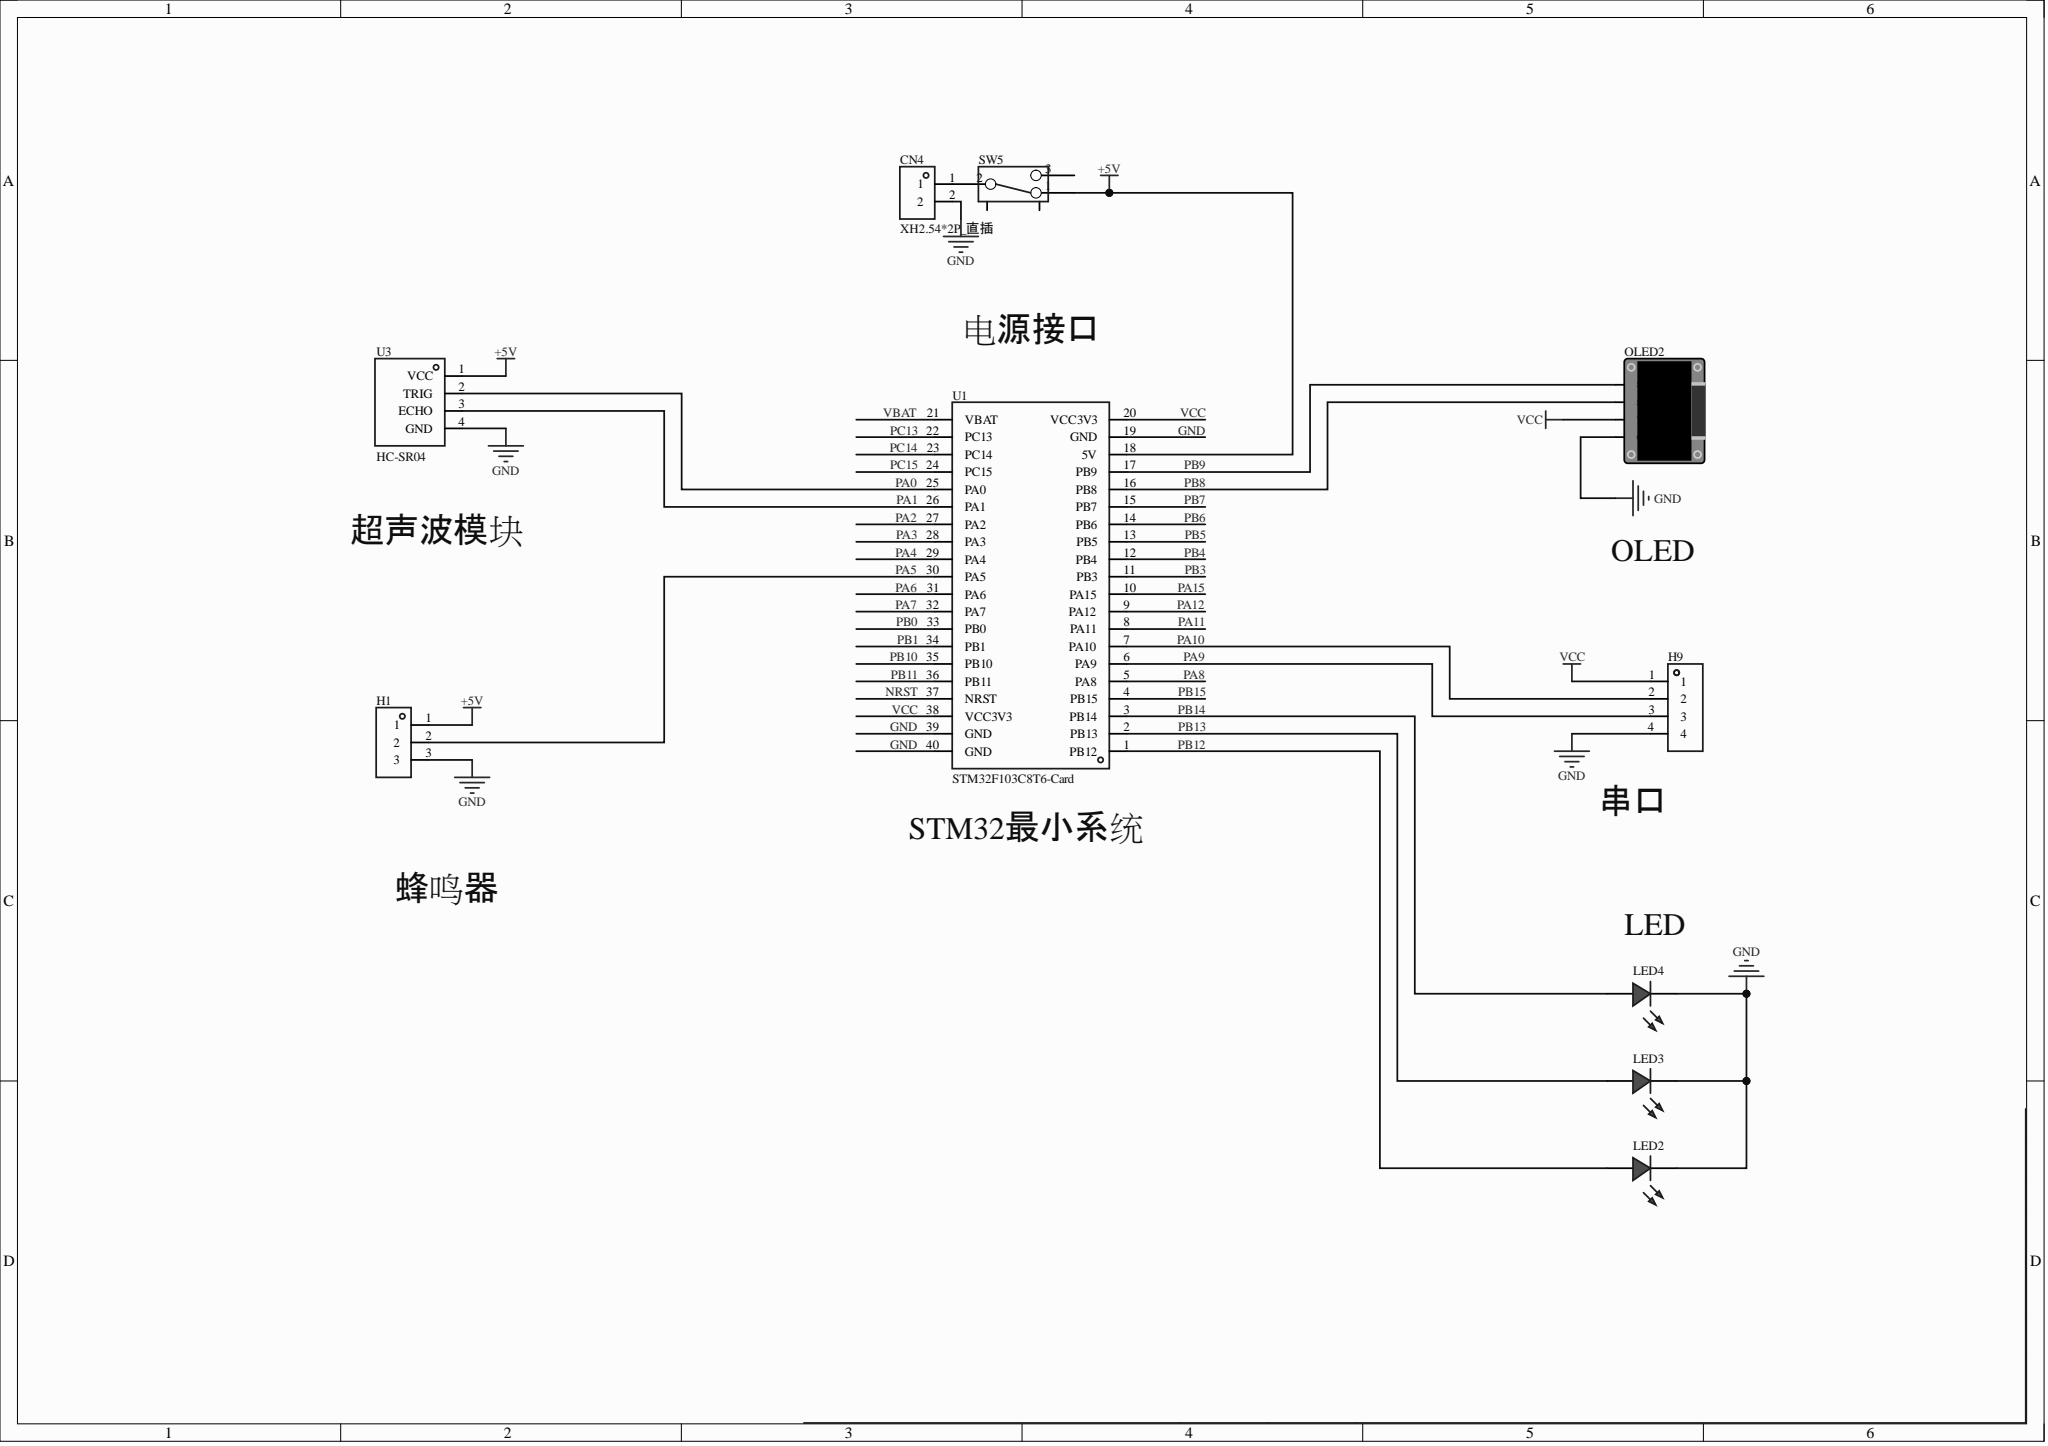Circuit board | Altium Designer | 10 parts | 14 nets
Bill of materials:
Comment,Description,Designator,Footprint,LibRef,Quantity
"XH2.54*2P_直插","","CN4","CONN-TH_2P-P2.50-XH2.54-2P","XH2.54*2P_直插","1"
"","","H1","HDR-TH_3P-P2.54-V-F","HDR-F_2.54_1x3P","1"
"","","H9","HDR-TH_4P-P2.54-V-F","HDR-F_2.54_1x4P","1"
"","","LED2, LED3, LED4","LED_TH-3mm","LED_TH-R_3mm","3"
"","","OLED2","0.96OLED_4P","0.96OLED模块_4P","1"
"","","SW5","拨动开关","拨动开关_正","1"
"STM32F103C8T6-Card","","U1","CONN-TH_L53.3-W22.9_STM32F103C8T6-CARD","STM32F103C8T6-Card","1"
"HC-SR04","","U3","TH_HC-SR04V","HC-SR04","1"
Netlist (Protel format):
[
CN4
CONN-TH_2P-P2.50-XH2.54-2P
XH2.54*2P_直插



]
[
H1
HDR-TH_3P-P2.54-V-F




]
[
H9
HDR-TH_4P-P2.54-V-F




]
[
LED2
LED_TH-3mm




]
[
LED3
LED_TH-3mm




]
[
LED4
LED_TH-3mm




]
[
OLED2
0.96OLED_4P




]
[
SW5
拨动开关




]
[
U1
CONN-TH_L53.3-W22.9_STM32F103C8T6-CARD
STM32F103C8T6-Card



]
[
U3
TH_HC-SR04V
HC-SR04



]
(
VCC
H9-1
OLED2-2
U1-20
U1-38
)
(
PB14
LED4-1
U1-3
)
(
PB13
LED3-1
U1-2
)
(
PB12
LED2-1
U1-1
)
(
PB9
OLED2-4
U1-17
)
(
PB8
OLED2-3
U1-16
)
(
PA10
H9-2
U1-7
)
(
PA9
H9-3
U1-6
)
(
PA5
H1-2
U1-30
)
(
PA1
U1-26
U3-3
)
(
PA0
U1-25
U3-2
)
(
NetCN4_1
CN4-1
SW5-2
)
(
GND
CN4-2
H1-3
H9-4
LED2-2
LED3-2
LED4-2
OLED2-1
U1-19
U1-39
U1-40
U3-4
)
(
+5V
H1-1
SW5-1
U1-18
U3-1
)